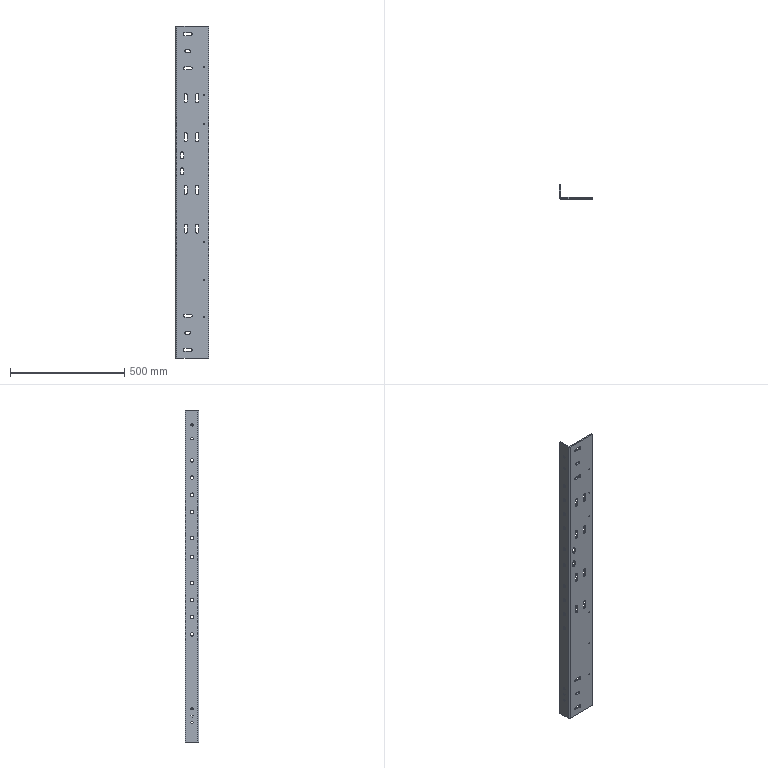Part | SolidWorks | features ICE 4, Cut 1, EdgeFlange 1, FlatPattern 1, SMBaseFlange 1, SheetMetal 1 | 1 solid | 131 faces | box 145 x 60 x 1450 mm | volume 1662951 mm3 | cylinder 84 | plane 47 | commonest cylinder face diameters 14 x24 15 x20 13 x14 4.5 x12 10 x8 11 x4